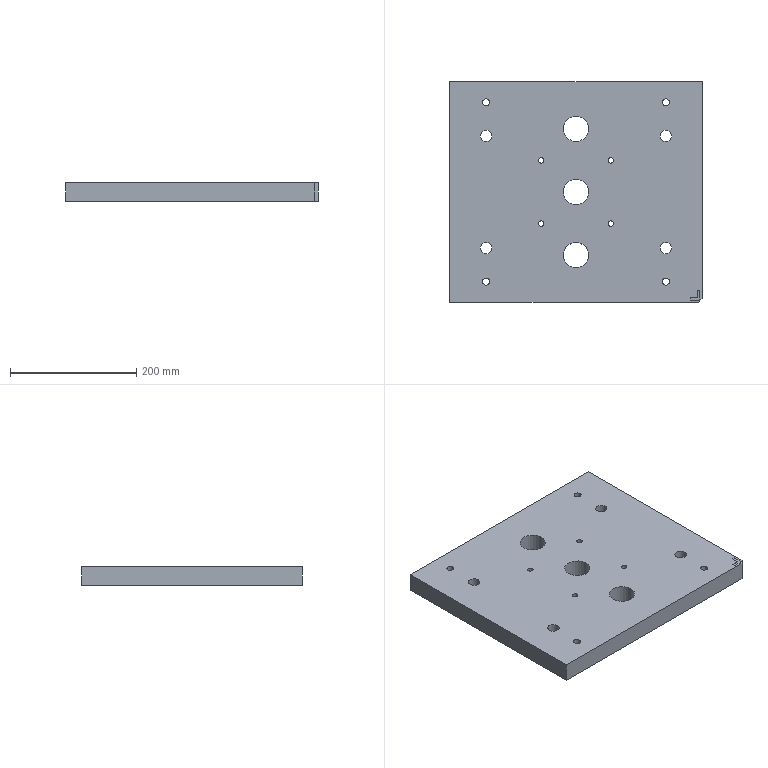Part | NX | features BD 2 | 1 solid | 56 faces | box 400 x 350 x 30 mm | volume 4007545 mm3 | cylinder 27 | plane 26 | cone 3 | commonest cylinder face diameters 18 x8 8.5 x4 11 x4 14 x4 26 x4 40 x3
STEP:
#1=CARTESIAN_POINT('',(48.,50.,-270.5));
#2=VERTEX_POINT('',#1);
#3=CARTESIAN_POINT('',(55.,50.,-270.5));
#4=DIRECTION('',(0.,0.,1.));
#5=DIRECTION('',(-1.,0.,0.));
#6=AXIS2_PLACEMENT_3D('',#3,#4,#5);
#7=CIRCLE('',#6,7.);
#8=EDGE_CURVE('',#2,#2,#7,.T.);
#9=ORIENTED_EDGE('',*,*,#8,.T.);
#10=EDGE_LOOP('',(#9));
#11=FACE_BOUND('',#10,.T.);
#12=CARTESIAN_POINT('',(-48.,-50.,-270.5));
#13=VERTEX_POINT('',#12);
#14=CARTESIAN_POINT('',(-55.,-50.,-270.5));
#15=DIRECTION('',(0.,0.,1.));
#16=DIRECTION('',(1.,0.,0.));
#17=AXIS2_PLACEMENT_3D('',#14,#15,#16);
#18=CIRCLE('',#17,7.);
#19=EDGE_CURVE('',#13,#13,#18,.T.);
#20=ORIENTED_EDGE('',*,*,#19,.T.);
#21=EDGE_LOOP('',(#20));
#22=FACE_BOUND('',#21,.T.);
#23=CARTESIAN_POINT('',(-21.,-100.,-270.5));
#24=VERTEX_POINT('',#23);
#25=CARTESIAN_POINT('',(0.,-100.,-270.5));
#26=DIRECTION('',(0.,0.,-1.));
#27=DIRECTION('',(-1.,0.,0.));
#28=AXIS2_PLACEMENT_3D('',#25,#26,#27);
#29=CIRCLE('',#28,21.);
#30=EDGE_CURVE('',#24,#24,#29,.F.);
#31=ORIENTED_EDGE('',*,*,#30,.T.);
#32=EDGE_LOOP('',(#31));
#33=FACE_BOUND('',#32,.T.);
#34=CARTESIAN_POINT('',(-21.,100.,-270.5));
#35=VERTEX_POINT('',#34);
#36=CARTESIAN_POINT('',(0.,100.,-270.5));
#37=DIRECTION('',(0.,0.,-1.));
#38=DIRECTION('',(-1.,0.,0.));
#39=AXIS2_PLACEMENT_3D('',#36,#37,#38);
#40=CIRCLE('',#39,21.);
#41=EDGE_CURVE('',#35,#35,#40,.F.);
#42=ORIENTED_EDGE('',*,*,#41,.T.);
#43=EDGE_LOOP('',(#42));
#44=FACE_BOUND('',#43,.T.);
#45=CARTESIAN_POINT('',(-21.,0.,-270.5));
#46=VERTEX_POINT('',#45);
#47=CARTESIAN_POINT('',(0.,0.,-270.5));
#48=DIRECTION('',(0.,0.,-1.));
#49=DIRECTION('',(-1.,0.,0.));
#50=AXIS2_PLACEMENT_3D('',#47,#48,#49);
#51=CIRCLE('',#50,21.);
#52=EDGE_CURVE('',#46,#46,#51,.F.);
#53=ORIENTED_EDGE('',*,*,#52,.T.);
#54=EDGE_LOOP('',(#53));
#55=FACE_BOUND('',#54,.T.);
#56=CARTESIAN_POINT('',(-151.5,-142.,-270.5));
#57=VERTEX_POINT('',#56);
#58=CARTESIAN_POINT('',(-142.5,-142.,-270.5));
#59=DIRECTION('',(0.,0.,1.));
#60=DIRECTION('',(-1.,0.,0.));
#61=AXIS2_PLACEMENT_3D('',#58,#59,#60);
#62=CIRCLE('',#61,9.);
#63=EDGE_CURVE('',#57,#57,#62,.T.);
#64=ORIENTED_EDGE('',*,*,#63,.T.);
#65=EDGE_LOOP('',(#64));
#66=FACE_BOUND('',#65,.T.);
#67=CARTESIAN_POINT('',(151.5,-142.,-270.5));
#68=VERTEX_POINT('',#67);
#69=CARTESIAN_POINT('',(142.5,-142.,-270.5));
#70=DIRECTION('',(0.,0.,1.));
#71=DIRECTION('',(1.,0.,0.));
#72=AXIS2_PLACEMENT_3D('',#69,#70,#71);
#73=CIRCLE('',#72,9.);
#74=EDGE_CURVE('',#68,#68,#73,.T.);
#75=ORIENTED_EDGE('',*,*,#74,.T.);
#76=EDGE_LOOP('',(#75));
#77=FACE_BOUND('',#76,.T.);
#78=CARTESIAN_POINT('',(-155.5,-89.,-270.5));
#79=VERTEX_POINT('',#78);
#80=CARTESIAN_POINT('',(-142.5,-89.,-270.5));
#81=DIRECTION('',(0.,0.,1.));
#82=DIRECTION('',(-1.,0.,0.));
#83=AXIS2_PLACEMENT_3D('',#80,#81,#82);
#84=CIRCLE('',#83,13.);
#85=EDGE_CURVE('',#79,#79,#84,.T.);
#86=ORIENTED_EDGE('',*,*,#85,.T.);
#87=EDGE_LOOP('',(#86));
#88=FACE_BOUND('',#87,.T.);
#89=CARTESIAN_POINT('',(155.5,89.,-270.5));
#90=VERTEX_POINT('',#89);
#91=CARTESIAN_POINT('',(142.5,89.,-270.5));
#92=DIRECTION('',(0.,0.,1.));
#93=DIRECTION('',(1.,0.,0.));
#94=AXIS2_PLACEMENT_3D('',#91,#92,#93);
#95=CIRCLE('',#94,13.);
#96=EDGE_CURVE('',#90,#90,#95,.T.);
#97=ORIENTED_EDGE('',*,*,#96,.T.);
#98=EDGE_LOOP('',(#97));
#99=FACE_BOUND('',#98,.T.);
#100=CARTESIAN_POINT('',(200.,-169.,-270.5));
#101=VERTEX_POINT('',#100);
#102=CARTESIAN_POINT('',(200.,175.,-270.5));
#103=VERTEX_POINT('',#102);
#104=CARTESIAN_POINT('',(200.,0.,-270.5));
#105=DIRECTION('',(0.,1.,0.));
#106=VECTOR('',#105,1000.);
#107=LINE('',#104,#106);
#108=EDGE_CURVE('',#101,#103,#107,.T.);
#109=ORIENTED_EDGE('',*,*,#108,.F.);
#110=CARTESIAN_POINT('',(194.,-175.,-270.5));
#111=VERTEX_POINT('',#110);
#112=CARTESIAN_POINT('',(184.5,-184.5,-270.5));
#113=DIRECTION('',(0.7071,0.7071,0.));
#114=VECTOR('',#113,1000.);
#115=LINE('',#112,#114);
#116=EDGE_CURVE('',#101,#111,#115,.F.);
#117=ORIENTED_EDGE('',*,*,#116,.T.);
#118=CARTESIAN_POINT('',(-200.,-175.,-270.5));
#119=VERTEX_POINT('',#118);
#120=CARTESIAN_POINT('',(0.,-175.,-270.5));
#121=DIRECTION('',(1.,0.,0.));
#122=VECTOR('',#121,1000.);
#123=LINE('',#120,#122);
#124=EDGE_CURVE('',#119,#111,#123,.T.);
#125=ORIENTED_EDGE('',*,*,#124,.F.);
#126=CARTESIAN_POINT('',(-200.,175.,-270.5));
#127=VERTEX_POINT('',#126);
#128=CARTESIAN_POINT('',(-200.,0.,-270.5));
#129=DIRECTION('',(0.,-1.,0.));
#130=VECTOR('',#129,1000.);
#131=LINE('',#128,#130);
#132=EDGE_CURVE('',#127,#119,#131,.T.);
#133=ORIENTED_EDGE('',*,*,#132,.F.);
#134=CARTESIAN_POINT('',(0.,175.,-270.5));
#135=DIRECTION('',(-1.,0.,0.));
#136=VECTOR('',#135,1000.);
#137=LINE('',#134,#136);
#138=EDGE_CURVE('',#103,#127,#137,.T.);
#139=ORIENTED_EDGE('',*,*,#138,.F.);
#140=EDGE_LOOP('',(#109,#117,#125,#133,#139));
#141=FACE_BOUND('',#140,.T.);
#142=CARTESIAN_POINT('',(155.5,-89.,-270.5));
#143=VERTEX_POINT('',#142);
#144=CARTESIAN_POINT('',(142.5,-89.,-270.5));
#145=DIRECTION('',(0.,0.,1.));
#146=DIRECTION('',(1.,0.,0.));
#147=AXIS2_PLACEMENT_3D('',#144,#145,#146);
#148=CIRCLE('',#147,13.);
#149=EDGE_CURVE('',#143,#143,#148,.T.);
#150=ORIENTED_EDGE('',*,*,#149,.T.);
#151=EDGE_LOOP('',(#150));
#152=FACE_BOUND('',#151,.T.);
#153=CARTESIAN_POINT('',(-129.5,89.,-270.5));
#154=VERTEX_POINT('',#153);
#155=CARTESIAN_POINT('',(-142.5,89.,-270.5));
#156=DIRECTION('',(0.,0.,1.));
#157=DIRECTION('',(1.,0.,0.));
#158=AXIS2_PLACEMENT_3D('',#155,#156,#157);
#159=CIRCLE('',#158,13.);
#160=EDGE_CURVE('',#154,#154,#159,.T.);
#161=ORIENTED_EDGE('',*,*,#160,.T.);
#162=EDGE_LOOP('',(#161));
#163=FACE_BOUND('',#162,.T.);
#164=CARTESIAN_POINT('',(151.5,142.,-270.5));
#165=VERTEX_POINT('',#164);
#166=CARTESIAN_POINT('',(142.5,142.,-270.5));
#167=DIRECTION('',(0.,0.,1.));
#168=DIRECTION('',(1.,0.,0.));
#169=AXIS2_PLACEMENT_3D('',#166,#167,#168);
#170=CIRCLE('',#169,9.);
#171=EDGE_CURVE('',#165,#165,#170,.T.);
#172=ORIENTED_EDGE('',*,*,#171,.T.);
#173=EDGE_LOOP('',(#172));
#174=FACE_BOUND('',#173,.T.);
#175=CARTESIAN_POINT('',(-133.5,142.,-270.5));
#176=VERTEX_POINT('',#175);
#177=CARTESIAN_POINT('',(-142.5,142.,-270.5));
#178=DIRECTION('',(0.,0.,1.));
#179=DIRECTION('',(1.,0.,0.));
#180=AXIS2_PLACEMENT_3D('',#177,#178,#179);
#181=CIRCLE('',#180,9.);
#182=EDGE_CURVE('',#176,#176,#181,.T.);
#183=ORIENTED_EDGE('',*,*,#182,.T.);
#184=EDGE_LOOP('',(#183));
#185=FACE_BOUND('',#184,.T.);
#186=CARTESIAN_POINT('',(62.,-50.,-270.5));
#187=VERTEX_POINT('',#186);
#188=CARTESIAN_POINT('',(55.,-50.,-270.5));
#189=DIRECTION('',(0.,0.,1.));
#190=DIRECTION('',(1.,0.,0.));
#191=AXIS2_PLACEMENT_3D('',#188,#189,#190);
#192=CIRCLE('',#191,7.);
#193=EDGE_CURVE('',#187,#187,#192,.T.);
#194=ORIENTED_EDGE('',*,*,#193,.T.);
#195=EDGE_LOOP('',(#194));
#196=FACE_BOUND('',#195,.T.);
#197=CARTESIAN_POINT('',(-48.,50.,-270.5));
#198=VERTEX_POINT('',#197);
#199=CARTESIAN_POINT('',(-55.,50.,-270.5));
#200=DIRECTION('',(0.,0.,1.));
#201=DIRECTION('',(1.,0.,0.));
#202=AXIS2_PLACEMENT_3D('',#199,#200,#201);
#203=CIRCLE('',#202,7.);
#204=EDGE_CURVE('',#198,#198,#203,.T.);
#205=ORIENTED_EDGE('',*,*,#204,.T.);
#206=EDGE_LOOP('',(#205));
#207=FACE_BOUND('',#206,.T.);
#208=CARTESIAN_POINT('',(0.,0.,-270.5));
#209=DIRECTION('',(0.,0.,-1.));
#210=DIRECTION('',(-1.,0.,0.));
#211=AXIS2_PLACEMENT_3D('',#208,#209,#210);
#212=PLANE('',#211);
#213=ADVANCED_FACE('',(#11,#22,#33,#44,#55,#66,#77,#88,#99,#141,#152,#163,#174,#185,#196,#207),#212,.T.);
#214=CARTESIAN_POINT('',(50.75,50.,-240.5));
#215=VERTEX_POINT('',#214);
#216=CARTESIAN_POINT('',(55.,50.,-240.5));
#217=DIRECTION('',(0.,0.,-1.));
#218=DIRECTION('',(-1.,0.,0.));
#219=AXIS2_PLACEMENT_3D('',#216,#217,#218);
#220=CIRCLE('',#219,4.25);
#221=EDGE_CURVE('',#215,#215,#220,.T.);
#222=ORIENTED_EDGE('',*,*,#221,.T.);
#223=EDGE_LOOP('',(#222));
#224=FACE_BOUND('',#223,.T.);
#225=CARTESIAN_POINT('',(-50.75,-50.,-240.5));
#226=VERTEX_POINT('',#225);
#227=CARTESIAN_POINT('',(-55.,-50.,-240.5));
#228=DIRECTION('',(0.,0.,-1.));
#229=DIRECTION('',(1.,0.,0.));
#230=AXIS2_PLACEMENT_3D('',#227,#228,#229);
#231=CIRCLE('',#230,4.25);
#232=EDGE_CURVE('',#226,#226,#231,.T.);
#233=ORIENTED_EDGE('',*,*,#232,.T.);
#234=EDGE_LOOP('',(#233));
#235=FACE_BOUND('',#234,.T.);
#236=CARTESIAN_POINT('',(20.,-100.,-240.5));
#237=VERTEX_POINT('',#236);
#238=CARTESIAN_POINT('',(0.,-100.,-240.5));
#239=DIRECTION('',(0.,0.,1.));
#240=DIRECTION('',(1.,0.,0.));
#241=AXIS2_PLACEMENT_3D('',#238,#239,#240);
#242=CIRCLE('',#241,20.);
#243=EDGE_CURVE('',#237,#237,#242,.T.);
#244=ORIENTED_EDGE('',*,*,#243,.F.);
#245=EDGE_LOOP('',(#244));
#246=FACE_BOUND('',#245,.T.);
#247=CARTESIAN_POINT('',(20.,100.,-240.5));
#248=VERTEX_POINT('',#247);
#249=CARTESIAN_POINT('',(0.,100.,-240.5));
#250=DIRECTION('',(0.,0.,1.));
#251=DIRECTION('',(1.,0.,0.));
#252=AXIS2_PLACEMENT_3D('',#249,#250,#251);
#253=CIRCLE('',#252,20.);
#254=EDGE_CURVE('',#248,#248,#253,.T.);
#255=ORIENTED_EDGE('',*,*,#254,.F.);
#256=EDGE_LOOP('',(#255));
#257=FACE_BOUND('',#256,.T.);
#258=CARTESIAN_POINT('',(-148.,-142.,-240.5));
#259=VERTEX_POINT('',#258);
#260=CARTESIAN_POINT('',(-142.5,-142.,-240.5));
#261=DIRECTION('',(0.,0.,-1.));
#262=DIRECTION('',(-1.,0.,0.));
#263=AXIS2_PLACEMENT_3D('',#260,#261,#262);
#264=CIRCLE('',#263,5.5);
#265=EDGE_CURVE('',#259,#259,#264,.T.);
#266=ORIENTED_EDGE('',*,*,#265,.T.);
#267=EDGE_LOOP('',(#266));
#268=FACE_BOUND('',#267,.T.);
#269=CARTESIAN_POINT('',(148.,-142.,-240.5));
#270=VERTEX_POINT('',#269);
#271=CARTESIAN_POINT('',(142.5,-142.,-240.5));
#272=DIRECTION('',(0.,0.,-1.));
#273=DIRECTION('',(1.,0.,0.));
#274=AXIS2_PLACEMENT_3D('',#271,#272,#273);
#275=CIRCLE('',#274,5.5);
#276=EDGE_CURVE('',#270,#270,#275,.T.);
#277=ORIENTED_EDGE('',*,*,#276,.T.);
#278=EDGE_LOOP('',(#277));
#279=FACE_BOUND('',#278,.T.);
#280=CARTESIAN_POINT('',(-151.5,-89.,-240.5));
#281=VERTEX_POINT('',#280);
#282=CARTESIAN_POINT('',(-142.5,-89.,-240.5));
#283=DIRECTION('',(0.,0.,-1.));
#284=DIRECTION('',(-1.,0.,0.));
#285=AXIS2_PLACEMENT_3D('',#282,#283,#284);
#286=CIRCLE('',#285,9.);
#287=EDGE_CURVE('',#281,#281,#286,.T.);
#288=ORIENTED_EDGE('',*,*,#287,.T.);
#289=EDGE_LOOP('',(#288));
#290=FACE_BOUND('',#289,.T.);
#291=CARTESIAN_POINT('',(151.5,89.,-240.5));
#292=VERTEX_POINT('',#291);
#293=CARTESIAN_POINT('',(142.5,89.,-240.5));
#294=DIRECTION('',(0.,0.,-1.));
#295=DIRECTION('',(1.,0.,0.));
#296=AXIS2_PLACEMENT_3D('',#293,#294,#295);
#297=CIRCLE('',#296,9.);
#298=EDGE_CURVE('',#292,#292,#297,.T.);
#299=ORIENTED_EDGE('',*,*,#298,.T.);
#300=EDGE_LOOP('',(#299));
#301=FACE_BOUND('',#300,.T.);
#302=CARTESIAN_POINT('',(192.5,-156.25,-240.5));
#303=VERTEX_POINT('',#302);
#304=CARTESIAN_POINT('',(192.5,-167.5,-240.5));
#305=VERTEX_POINT('',#304);
#306=CARTESIAN_POINT('',(192.5,-161.875,-240.5));
#307=DIRECTION('',(0.,-1.,0.));
#308=VECTOR('',#307,1000.);
#309=LINE('',#306,#308);
#310=EDGE_CURVE('',#303,#305,#309,.T.);
#311=ORIENTED_EDGE('',*,*,#310,.F.);
#312=CARTESIAN_POINT('',(196.25,-156.25,-240.5));
#313=VERTEX_POINT('',#312);
#314=CARTESIAN_POINT('',(188.75,-156.25,-240.5));
#315=DIRECTION('',(1.,0.,0.));
#316=VECTOR('',#315,1000.);
#317=LINE('',#314,#316);
#318=EDGE_CURVE('',#303,#313,#317,.T.);
#319=ORIENTED_EDGE('',*,*,#318,.T.);
#320=CARTESIAN_POINT('',(196.25,-171.25,-240.5));
#321=VERTEX_POINT('',#320);
#322=CARTESIAN_POINT('',(196.25,-163.75,-240.5));
#323=DIRECTION('',(0.,-1.,0.));
#324=VECTOR('',#323,1000.);
#325=LINE('',#322,#324);
#326=EDGE_CURVE('',#313,#321,#325,.T.);
#327=ORIENTED_EDGE('',*,*,#326,.T.);
#328=CARTESIAN_POINT('',(181.25,-171.25,-240.5));
#329=VERTEX_POINT('',#328);
#330=CARTESIAN_POINT('',(188.75,-171.25,-240.5));
#331=DIRECTION('',(-1.,0.,0.));
#332=VECTOR('',#331,1000.);
#333=LINE('',#330,#332);
#334=EDGE_CURVE('',#321,#329,#333,.T.);
#335=ORIENTED_EDGE('',*,*,#334,.T.);
#336=CARTESIAN_POINT('',(181.25,-167.5,-240.5));
#337=VERTEX_POINT('',#336);
#338=CARTESIAN_POINT('',(181.25,-163.75,-240.5));
#339=DIRECTION('',(0.,1.,0.));
#340=VECTOR('',#339,1000.);
#341=LINE('',#338,#340);
#342=EDGE_CURVE('',#329,#337,#341,.T.);
#343=ORIENTED_EDGE('',*,*,#342,.T.);
#344=CARTESIAN_POINT('',(186.875,-167.5,-240.5));
#345=DIRECTION('',(-1.,0.,0.));
#346=VECTOR('',#345,1000.);
#347=LINE('',#344,#346);
#348=EDGE_CURVE('',#305,#337,#347,.T.);
#349=ORIENTED_EDGE('',*,*,#348,.F.);
#350=EDGE_LOOP('',(#311,#319,#327,#335,#343,#349));
#351=FACE_BOUND('',#350,.T.);
#352=CARTESIAN_POINT('',(194.,-175.,-240.5));
#353=VERTEX_POINT('',#352);
#354=CARTESIAN_POINT('',(-200.,-175.,-240.5));
#355=VERTEX_POINT('',#354);
#356=CARTESIAN_POINT('',(0.,-175.,-240.5));
#357=DIRECTION('',(-1.,0.,0.));
#358=VECTOR('',#357,1000.);
#359=LINE('',#356,#358);
#360=EDGE_CURVE('',#353,#355,#359,.T.);
#361=ORIENTED_EDGE('',*,*,#360,.F.);
#362=CARTESIAN_POINT('',(200.,-169.,-240.5));
#363=VERTEX_POINT('',#362);
#364=CARTESIAN_POINT('',(184.5,-184.5,-240.5));
#365=DIRECTION('',(-0.7071,-0.7071,0.));
#366=VECTOR('',#365,1000.);
#367=LINE('',#364,#366);
#368=EDGE_CURVE('',#353,#363,#367,.F.);
#369=ORIENTED_EDGE('',*,*,#368,.T.);
#370=CARTESIAN_POINT('',(200.,175.,-240.5));
#371=VERTEX_POINT('',#370);
#372=CARTESIAN_POINT('',(200.,0.,-240.5));
#373=DIRECTION('',(0.,-1.,0.));
#374=VECTOR('',#373,1000.);
#375=LINE('',#372,#374);
#376=EDGE_CURVE('',#371,#363,#375,.T.);
#377=ORIENTED_EDGE('',*,*,#376,.F.);
#378=CARTESIAN_POINT('',(-200.,175.,-240.5));
#379=VERTEX_POINT('',#378);
#380=CARTESIAN_POINT('',(0.,175.,-240.5));
#381=DIRECTION('',(1.,0.,0.));
#382=VECTOR('',#381,1000.);
#383=LINE('',#380,#382);
#384=EDGE_CURVE('',#379,#371,#383,.T.);
#385=ORIENTED_EDGE('',*,*,#384,.F.);
#386=CARTESIAN_POINT('',(-200.,0.,-240.5));
#387=DIRECTION('',(0.,1.,0.));
#388=VECTOR('',#387,1000.);
#389=LINE('',#386,#388);
#390=EDGE_CURVE('',#355,#379,#389,.T.);
#391=ORIENTED_EDGE('',*,*,#390,.F.);
#392=EDGE_LOOP('',(#361,#369,#377,#385,#391));
#393=FACE_BOUND('',#392,.T.);
#394=CARTESIAN_POINT('',(151.5,-89.,-240.5));
#395=VERTEX_POINT('',#394);
#396=CARTESIAN_POINT('',(142.5,-89.,-240.5));
#397=DIRECTION('',(0.,0.,-1.));
#398=DIRECTION('',(1.,0.,0.));
#399=AXIS2_PLACEMENT_3D('',#396,#397,#398);
#400=CIRCLE('',#399,9.);
#401=EDGE_CURVE('',#395,#395,#400,.T.);
#402=ORIENTED_EDGE('',*,*,#401,.T.);
#403=EDGE_LOOP('',(#402));
#404=FACE_BOUND('',#403,.T.);
#405=CARTESIAN_POINT('',(-133.5,89.,-240.5));
#406=VERTEX_POINT('',#405);
#407=CARTESIAN_POINT('',(-142.5,89.,-240.5));
#408=DIRECTION('',(0.,0.,-1.));
#409=DIRECTION('',(1.,0.,0.));
#410=AXIS2_PLACEMENT_3D('',#407,#408,#409);
#411=CIRCLE('',#410,9.);
#412=EDGE_CURVE('',#406,#406,#411,.T.);
#413=ORIENTED_EDGE('',*,*,#412,.T.);
#414=EDGE_LOOP('',(#413));
#415=FACE_BOUND('',#414,.T.);
#416=CARTESIAN_POINT('',(148.,142.,-240.5));
#417=VERTEX_POINT('',#416);
#418=CARTESIAN_POINT('',(142.5,142.,-240.5));
#419=DIRECTION('',(0.,0.,-1.));
#420=DIRECTION('',(1.,0.,0.));
#421=AXIS2_PLACEMENT_3D('',#418,#419,#420);
#422=CIRCLE('',#421,5.5);
#423=EDGE_CURVE('',#417,#417,#422,.T.);
#424=ORIENTED_EDGE('',*,*,#423,.T.);
#425=EDGE_LOOP('',(#424));
#426=FACE_BOUND('',#425,.T.);
#427=CARTESIAN_POINT('',(-137.,142.,-240.5));
#428=VERTEX_POINT('',#427);
#429=CARTESIAN_POINT('',(-142.5,142.,-240.5));
#430=DIRECTION('',(0.,0.,-1.));
#431=DIRECTION('',(1.,0.,0.));
#432=AXIS2_PLACEMENT_3D('',#429,#430,#431);
#433=CIRCLE('',#432,5.5);
#434=EDGE_CURVE('',#428,#428,#433,.T.);
#435=ORIENTED_EDGE('',*,*,#434,.T.);
#436=EDGE_LOOP('',(#435));
#437=FACE_BOUND('',#436,.T.);
#438=CARTESIAN_POINT('',(20.,0.,-240.5));
#439=VERTEX_POINT('',#438);
#440=CARTESIAN_POINT('',(0.,0.,-240.5));
#441=DIRECTION('',(0.,0.,1.));
#442=DIRECTION('',(1.,0.,0.));
#443=AXIS2_PLACEMENT_3D('',#440,#441,#442);
#444=CIRCLE('',#443,20.);
#445=EDGE_CURVE('',#439,#439,#444,.F.);
#446=ORIENTED_EDGE('',*,*,#445,.T.);
#447=EDGE_LOOP('',(#446));
#448=FACE_BOUND('',#447,.T.);
#449=CARTESIAN_POINT('',(59.25,-50.,-240.5));
#450=VERTEX_POINT('',#449);
#451=CARTESIAN_POINT('',(55.,-50.,-240.5));
#452=DIRECTION('',(0.,0.,-1.));
#453=DIRECTION('',(1.,0.,0.));
#454=AXIS2_PLACEMENT_3D('',#451,#452,#453);
#455=CIRCLE('',#454,4.25);
#456=EDGE_CURVE('',#450,#450,#455,.T.);
#457=ORIENTED_EDGE('',*,*,#456,.T.);
#458=EDGE_LOOP('',(#457));
#459=FACE_BOUND('',#458,.T.);
#460=CARTESIAN_POINT('',(-50.75,50.,-240.5));
#461=VERTEX_POINT('',#460);
#462=CARTESIAN_POINT('',(-55.,50.,-240.5));
#463=DIRECTION('',(0.,0.,-1.));
#464=DIRECTION('',(1.,0.,0.));
#465=AXIS2_PLACEMENT_3D('',#462,#463,#464);
#466=CIRCLE('',#465,4.25);
#467=EDGE_CURVE('',#461,#461,#466,.T.);
#468=ORIENTED_EDGE('',*,*,#467,.T.);
#469=EDGE_LOOP('',(#468));
#470=FACE_BOUND('',#469,.T.);
#471=CARTESIAN_POINT('',(0.,0.,-240.5));
#472=DIRECTION('',(0.,0.,1.));
#473=DIRECTION('',(1.,0.,0.));
#474=AXIS2_PLACEMENT_3D('',#471,#472,#473);
#475=PLANE('',#474);
#476=ADVANCED_FACE('',(#224,#235,#246,#257,#268,#279,#290,#301,#351,#393,#404,#415,#426,#437,#448,#459,#470),#475,.T.);
#477=CARTESIAN_POINT('',(-20.,-100.,-269.5));
#478=VERTEX_POINT('',#477);
#479=CARTESIAN_POINT('',(0.,-100.,-269.5));
#480=DIRECTION('',(0.,0.,-1.));
#481=DIRECTION('',(-1.,0.,0.));
#482=AXIS2_PLACEMENT_3D('',#479,#480,#481);
#483=CIRCLE('',#482,20.);
#484=EDGE_CURVE('',#478,#478,#483,.T.);
#485=ORIENTED_EDGE('',*,*,#484,.T.);
#486=EDGE_LOOP('',(#485));
#487=FACE_BOUND('',#486,.T.);
#488=ORIENTED_EDGE('',*,*,#243,.T.);
#489=EDGE_LOOP('',(#488));
#490=FACE_BOUND('',#489,.T.);
#491=CARTESIAN_POINT('',(0.,-100.,-270.5));
#492=DIRECTION('',(0.,0.,1.));
#493=DIRECTION('',(1.,0.,0.));
#494=AXIS2_PLACEMENT_3D('',#491,#492,#493);
#495=CYLINDRICAL_SURFACE('',#494,20.);
#496=ADVANCED_FACE('',(#487,#490),#495,.F.);
#497=CARTESIAN_POINT('',(192.5,-167.5,-240.6));
#498=VERTEX_POINT('',#497);
#499=CARTESIAN_POINT('',(181.25,-167.5,-240.6));
#500=VERTEX_POINT('',#499);
#501=CARTESIAN_POINT('',(186.875,-167.5,-240.6));
#502=DIRECTION('',(1.,0.,0.));
#503=VECTOR('',#502,1000.);
#504=LINE('',#501,#503);
#505=EDGE_CURVE('',#498,#500,#504,.F.);
#506=ORIENTED_EDGE('',*,*,#505,.T.);
#507=CARTESIAN_POINT('',(181.25,-171.25,-240.6));
#508=VERTEX_POINT('',#507);
#509=CARTESIAN_POINT('',(181.25,-163.75,-240.6));
#510=DIRECTION('',(0.,-1.,0.));
#511=VECTOR('',#510,1000.);
#512=LINE('',#509,#511);
#513=EDGE_CURVE('',#508,#500,#512,.F.);
#514=ORIENTED_EDGE('',*,*,#513,.F.);
#515=CARTESIAN_POINT('',(196.25,-171.25,-240.6));
#516=VERTEX_POINT('',#515);
#517=CARTESIAN_POINT('',(188.75,-171.25,-240.6));
#518=DIRECTION('',(1.,0.,0.));
#519=VECTOR('',#518,1000.);
#520=LINE('',#517,#519);
#521=EDGE_CURVE('',#516,#508,#520,.F.);
#522=ORIENTED_EDGE('',*,*,#521,.F.);
#523=CARTESIAN_POINT('',(196.25,-156.25,-240.6));
#524=VERTEX_POINT('',#523);
#525=CARTESIAN_POINT('',(196.25,-163.75,-240.6));
#526=DIRECTION('',(0.,1.,0.));
#527=VECTOR('',#526,1000.);
#528=LINE('',#525,#527);
#529=EDGE_CURVE('',#524,#516,#528,.F.);
#530=ORIENTED_EDGE('',*,*,#529,.F.);
#531=CARTESIAN_POINT('',(192.5,-156.25,-240.6));
#532=VERTEX_POINT('',#531);
#533=CARTESIAN_POINT('',(188.75,-156.25,-240.6));
#534=DIRECTION('',(-1.,0.,0.));
#535=VECTOR('',#534,1000.);
#536=LINE('',#533,#535);
#537=EDGE_CURVE('',#532,#524,#536,.F.);
#538=ORIENTED_EDGE('',*,*,#537,.F.);
#539=CARTESIAN_POINT('',(192.5,-161.875,-240.6));
#540=DIRECTION('',(0.,1.,0.));
#541=VECTOR('',#540,1000.);
#542=LINE('',#539,#541);
#543=EDGE_CURVE('',#532,#498,#542,.F.);
#544=ORIENTED_EDGE('',*,*,#543,.T.);
#545=EDGE_LOOP('',(#506,#514,#522,#530,#538,#544));
#546=FACE_BOUND('',#545,.T.);
#547=CARTESIAN_POINT('',(188.75,-163.75,-240.6));
#548=DIRECTION('',(0.,0.,-1.));
#549=DIRECTION('',(-1.,0.,0.));
#550=AXIS2_PLACEMENT_3D('',#547,#548,#549);
#551=PLANE('',#550);
#552=ADVANCED_FACE('',(#546),#551,.F.);
#553=CARTESIAN_POINT('',(-137.,142.,-259.5));
#554=VERTEX_POINT('',#553);
#555=CARTESIAN_POINT('',(-142.5,142.,-259.5));
#556=DIRECTION('',(0.,0.,1.));
#557=DIRECTION('',(1.,0.,0.));
#558=AXIS2_PLACEMENT_3D('',#555,#556,#557);
#559=CIRCLE('',#558,5.5);
#560=EDGE_CURVE('',#554,#554,#559,.T.);
#561=ORIENTED_EDGE('',*,*,#560,.T.);
#562=EDGE_LOOP('',(#561));
#563=FACE_BOUND('',#562,.T.);
#564=CARTESIAN_POINT('',(-133.5,142.,-259.5));
#565=VERTEX_POINT('',#564);
#566=CARTESIAN_POINT('',(-142.5,142.,-259.5));
#567=DIRECTION('',(0.,0.,-1.));
#568=DIRECTION('',(1.,0.,0.));
#569=AXIS2_PLACEMENT_3D('',#566,#567,#568);
#570=CIRCLE('',#569,9.);
#571=EDGE_CURVE('',#565,#565,#570,.F.);
#572=ORIENTED_EDGE('',*,*,#571,.F.);
#573=EDGE_LOOP('',(#572));
#574=FACE_BOUND('',#573,.T.);
#575=CARTESIAN_POINT('',(-142.5,142.,-259.5));
#576=DIRECTION('',(0.,0.,1.));
#577=DIRECTION('',(1.,0.,0.));
#578=AXIS2_PLACEMENT_3D('',#575,#576,#577);
#579=PLANE('',#578);
#580=ADVANCED_FACE('',(#563,#574),#579,.F.);
#581=CARTESIAN_POINT('',(148.,142.,-259.5));
#582=VERTEX_POINT('',#581);
#583=CARTESIAN_POINT('',(142.5,142.,-259.5));
#584=DIRECTION('',(0.,0.,1.));
#585=DIRECTION('',(1.,0.,0.));
#586=AXIS2_PLACEMENT_3D('',#583,#584,#585);
#587=CIRCLE('',#586,5.5);
#588=EDGE_CURVE('',#582,#582,#587,.T.);
#589=ORIENTED_EDGE('',*,*,#588,.T.);
#590=EDGE_LOOP('',(#589));
#591=FACE_BOUND('',#590,.T.);
#592=CARTESIAN_POINT('',(151.5,142.,-259.5));
#593=VERTEX_POINT('',#592);
#594=CARTESIAN_POINT('',(142.5,142.,-259.5));
#595=DIRECTION('',(0.,0.,-1.));
#596=DIRECTION('',(1.,0.,0.));
#597=AXIS2_PLACEMENT_3D('',#594,#595,#596);
#598=CIRCLE('',#597,9.);
#599=EDGE_CURVE('',#593,#593,#598,.F.);
#600=ORIENTED_EDGE('',*,*,#599,.F.);
#601=EDGE_LOOP('',(#600));
#602=FACE_BOUND('',#601,.T.);
#603=CARTESIAN_POINT('',(142.5,142.,-259.5));
#604=DIRECTION('',(0.,0.,1.));
#605=DIRECTION('',(1.,0.,0.));
#606=AXIS2_PLACEMENT_3D('',#603,#604,#605);
#607=PLANE('',#606);
#608=ADVANCED_FACE('',(#591,#602),#607,.F.);
#609=CARTESIAN_POINT('',(-133.5,89.,-253.));
#610=VERTEX_POINT('',#609);
#611=CARTESIAN_POINT('',(-142.5,89.,-253.));
#612=DIRECTION('',(0.,0.,1.));
#613=DIRECTION('',(1.,0.,0.));
#614=AXIS2_PLACEMENT_3D('',#611,#612,#613);
#615=CIRCLE('',#614,9.);
#616=EDGE_CURVE('',#610,#610,#615,.T.);
#617=ORIENTED_EDGE('',*,*,#616,.T.);
#618=EDGE_LOOP('',(#617));
#619=FACE_BOUND('',#618,.T.);
#620=CARTESIAN_POINT('',(-129.5,89.,-253.));
#621=VERTEX_POINT('',#620);
#622=CARTESIAN_POINT('',(-142.5,89.,-253.));
#623=DIRECTION('',(0.,0.,-1.));
#624=DIRECTION('',(1.,0.,0.));
#625=AXIS2_PLACEMENT_3D('',#622,#623,#624);
#626=CIRCLE('',#625,13.);
#627=EDGE_CURVE('',#621,#621,#626,.F.);
#628=ORIENTED_EDGE('',*,*,#627,.F.);
#629=EDGE_LOOP('',(#628));
#630=FACE_BOUND('',#629,.T.);
#631=CARTESIAN_POINT('',(-142.5,89.,-253.));
#632=DIRECTION('',(0.,0.,1.));
#633=DIRECTION('',(1.,0.,0.));
#634=AXIS2_PLACEMENT_3D('',#631,#632,#633);
#635=PLANE('',#634);
#636=ADVANCED_FACE('',(#619,#630),#635,.F.);
#637=CARTESIAN_POINT('',(151.5,-89.,-253.));
#638=VERTEX_POINT('',#637);
#639=CARTESIAN_POINT('',(142.5,-89.,-253.));
#640=DIRECTION('',(0.,0.,1.));
#641=DIRECTION('',(1.,0.,0.));
#642=AXIS2_PLACEMENT_3D('',#639,#640,#641);
#643=CIRCLE('',#642,9.);
#644=EDGE_CURVE('',#638,#638,#643,.T.);
#645=ORIENTED_EDGE('',*,*,#644,.T.);
#646=EDGE_LOOP('',(#645));
#647=FACE_BOUND('',#646,.T.);
#648=CARTESIAN_POINT('',(155.5,-89.,-253.));
#649=VERTEX_POINT('',#648);
#650=CARTESIAN_POINT('',(142.5,-89.,-253.));
#651=DIRECTION('',(0.,0.,-1.));
#652=DIRECTION('',(1.,0.,0.));
#653=AXIS2_PLACEMENT_3D('',#650,#651,#652);
#654=CIRCLE('',#653,13.);
#655=EDGE_CURVE('',#649,#649,#654,.F.);
#656=ORIENTED_EDGE('',*,*,#655,.F.);
#657=EDGE_LOOP('',(#656));
#658=FACE_BOUND('',#657,.T.);
#659=CARTESIAN_POINT('',(142.5,-89.,-253.));
#660=DIRECTION('',(0.,0.,1.));
#661=DIRECTION('',(1.,0.,0.));
#662=AXIS2_PLACEMENT_3D('',#659,#660,#661);
#663=PLANE('',#662);
#664=ADVANCED_FACE('',(#647,#658),#663,.F.);
#665=CARTESIAN_POINT('',(151.5,89.,-253.));
#666=VERTEX_POINT('',#665);
#667=CARTESIAN_POINT('',(142.5,89.,-253.));
#668=DIRECTION('',(0.,0.,1.));
#669=DIRECTION('',(1.,0.,0.));
#670=AXIS2_PLACEMENT_3D('',#667,#668,#669);
#671=CIRCLE('',#670,9.);
#672=EDGE_CURVE('',#666,#666,#671,.T.);
#673=ORIENTED_EDGE('',*,*,#672,.T.);
#674=EDGE_LOOP('',(#673));
#675=FACE_BOUND('',#674,.T.);
#676=CARTESIAN_POINT('',(155.5,89.,-253.));
#677=VERTEX_POINT('',#676);
#678=CARTESIAN_POINT('',(142.5,89.,-253.));
#679=DIRECTION('',(0.,0.,-1.));
#680=DIRECTION('',(1.,0.,0.));
#681=AXIS2_PLACEMENT_3D('',#678,#679,#680);
#682=CIRCLE('',#681,13.);
#683=EDGE_CURVE('',#677,#677,#682,.F.);
#684=ORIENTED_EDGE('',*,*,#683,.F.);
#685=EDGE_LOOP('',(#684));
#686=FACE_BOUND('',#685,.T.);
#687=CARTESIAN_POINT('',(142.5,89.,-253.));
#688=DIRECTION('',(0.,0.,1.));
#689=DIRECTION('',(1.,0.,0.));
#690=AXIS2_PLACEMENT_3D('',#687,#688,#689);
#691=PLANE('',#690);
#692=ADVANCED_FACE('',(#675,#686),#691,.F.);
#693=CARTESIAN_POINT('',(-151.5,-89.,-253.));
#694=VERTEX_POINT('',#693);
#695=CARTESIAN_POINT('',(-142.5,-89.,-253.));
#696=DIRECTION('',(0.,0.,1.));
#697=DIRECTION('',(-1.,0.,0.));
#698=AXIS2_PLACEMENT_3D('',#695,#696,#697);
#699=CIRCLE('',#698,9.);
#700=EDGE_CURVE('',#694,#694,#699,.T.);
#701=ORIENTED_EDGE('',*,*,#700,.T.);
#702=EDGE_LOOP('',(#701));
#703=FACE_BOUND('',#702,.T.);
#704=CARTESIAN_POINT('',(-155.5,-89.,-253.));
#705=VERTEX_POINT('',#704);
#706=CARTESIAN_POINT('',(-142.5,-89.,-253.));
#707=DIRECTION('',(0.,0.,-1.));
#708=DIRECTION('',(-1.,0.,0.));
#709=AXIS2_PLACEMENT_3D('',#706,#707,#708);
#710=CIRCLE('',#709,13.);
#711=EDGE_CURVE('',#705,#705,#710,.F.);
#712=ORIENTED_EDGE('',*,*,#711,.F.);
#713=EDGE_LOOP('',(#712));
#714=FACE_BOUND('',#713,.T.);
#715=CARTESIAN_POINT('',(-142.5,-89.,-253.));
#716=DIRECTION('',(0.,0.,1.));
#717=DIRECTION('',(-1.,0.,0.));
#718=AXIS2_PLACEMENT_3D('',#715,#716,#717);
#719=PLANE('',#718);
#720=ADVANCED_FACE('',(#703,#714),#719,.F.);
#721=CARTESIAN_POINT('',(148.,-142.,-259.5));
#722=VERTEX_POINT('',#721);
#723=CARTESIAN_POINT('',(142.5,-142.,-259.5));
#724=DIRECTION('',(0.,0.,1.));
#725=DIRECTION('',(1.,0.,0.));
#726=AXIS2_PLACEMENT_3D('',#723,#724,#725);
#727=CIRCLE('',#726,5.5);
#728=EDGE_CURVE('',#722,#722,#727,.T.);
#729=ORIENTED_EDGE('',*,*,#728,.T.);
#730=EDGE_LOOP('',(#729));
#731=FACE_BOUND('',#730,.T.);
#732=CARTESIAN_POINT('',(151.5,-142.,-259.5));
#733=VERTEX_POINT('',#732);
#734=CARTESIAN_POINT('',(142.5,-142.,-259.5));
#735=DIRECTION('',(0.,0.,-1.));
#736=DIRECTION('',(1.,0.,0.));
#737=AXIS2_PLACEMENT_3D('',#734,#735,#736);
#738=CIRCLE('',#737,9.);
#739=EDGE_CURVE('',#733,#733,#738,.F.);
#740=ORIENTED_EDGE('',*,*,#739,.F.);
#741=EDGE_LOOP('',(#740));
#742=FACE_BOUND('',#741,.T.);
#743=CARTESIAN_POINT('',(142.5,-142.,-259.5));
#744=DIRECTION('',(0.,0.,1.));
#745=DIRECTION('',(1.,0.,0.));
#746=AXIS2_PLACEMENT_3D('',#743,#744,#745);
#747=PLANE('',#746);
#748=ADVANCED_FACE('',(#731,#742),#747,.F.);
#749=CARTESIAN_POINT('',(-148.,-142.,-259.5));
#750=VERTEX_POINT('',#749);
#751=CARTESIAN_POINT('',(-142.5,-142.,-259.5));
#752=DIRECTION('',(0.,0.,1.));
#753=DIRECTION('',(-1.,0.,0.));
#754=AXIS2_PLACEMENT_3D('',#751,#752,#753);
#755=CIRCLE('',#754,5.5);
#756=EDGE_CURVE('',#750,#750,#755,.T.);
#757=ORIENTED_EDGE('',*,*,#756,.T.);
#758=EDGE_LOOP('',(#757));
#759=FACE_BOUND('',#758,.T.);
#760=CARTESIAN_POINT('',(-151.5,-142.,-259.5));
#761=VERTEX_POINT('',#760);
#762=CARTESIAN_POINT('',(-142.5,-142.,-259.5));
#763=DIRECTION('',(0.,0.,-1.));
#764=DIRECTION('',(-1.,0.,0.));
#765=AXIS2_PLACEMENT_3D('',#762,#763,#764);
#766=CIRCLE('',#765,9.);
#767=EDGE_CURVE('',#761,#761,#766,.F.);
#768=ORIENTED_EDGE('',*,*,#767,.F.);
#769=EDGE_LOOP('',(#768));
#770=FACE_BOUND('',#769,.T.);
#771=CARTESIAN_POINT('',(-142.5,-142.,-259.5));
#772=DIRECTION('',(0.,0.,1.));
#773=DIRECTION('',(-1.,0.,0.));
#774=AXIS2_PLACEMENT_3D('',#771,#772,#773);
#775=PLANE('',#774);
#776=ADVANCED_FACE('',(#759,#770),#775,.F.);
#777=CARTESIAN_POINT('',(-20.,0.,-269.5));
#778=VERTEX_POINT('',#777);
#779=CARTESIAN_POINT('',(0.,0.,-269.5));
#780=DIRECTION('',(0.,0.,-1.));
#781=DIRECTION('',(-1.,0.,0.));
#782=AXIS2_PLACEMENT_3D('',#779,#780,#781);
#783=CIRCLE('',#782,20.);
#784=EDGE_CURVE('',#778,#778,#783,.T.);
#785=ORIENTED_EDGE('',*,*,#784,.T.);
#786=EDGE_LOOP('',(#785));
#787=FACE_BOUND('',#786,.T.);
#788=ORIENTED_EDGE('',*,*,#445,.F.);
#789=EDGE_LOOP('',(#788));
#790=FACE_BOUND('',#789,.T.);
#791=CARTESIAN_POINT('',(0.,0.,-270.5));
#792=DIRECTION('',(0.,0.,1.));
#793=DIRECTION('',(1.,0.,0.));
#794=AXIS2_PLACEMENT_3D('',#791,#792,#793);
#795=CYLINDRICAL_SURFACE('',#794,20.);
#796=ADVANCED_FACE('',(#787,#790),#795,.F.);
#797=ORIENTED_EDGE('',*,*,#560,.F.);
#798=EDGE_LOOP('',(#797));
#799=FACE_BOUND('',#798,.T.);
#800=ORIENTED_EDGE('',*,*,#434,.F.);
#801=EDGE_LOOP('',(#800));
#802=FACE_BOUND('',#801,.T.);
#803=CARTESIAN_POINT('',(-142.5,142.,-270.5));
#804=DIRECTION('',(0.,0.,1.));
#805=DIRECTION('',(1.,0.,0.));
#806=AXIS2_PLACEMENT_3D('',#803,#804,#805);
#807=CYLINDRICAL_SURFACE('',#806,5.5);
#808=ADVANCED_FACE('',(#799,#802),#807,.F.);
#809=ORIENTED_EDGE('',*,*,#588,.F.);
#810=EDGE_LOOP('',(#809));
#811=FACE_BOUND('',#810,.T.);
#812=ORIENTED_EDGE('',*,*,#423,.F.);
#813=EDGE_LOOP('',(#812));
#814=FACE_BOUND('',#813,.T.);
#815=CARTESIAN_POINT('',(142.5,142.,-270.5));
#816=DIRECTION('',(0.,0.,1.));
#817=DIRECTION('',(1.,0.,0.));
#818=AXIS2_PLACEMENT_3D('',#815,#816,#817);
#819=CYLINDRICAL_SURFACE('',#818,5.5);
#820=ADVANCED_FACE('',(#811,#814),#819,.F.);
#821=ORIENTED_EDGE('',*,*,#616,.F.);
#822=EDGE_LOOP('',(#821));
#823=FACE_BOUND('',#822,.T.);
#824=ORIENTED_EDGE('',*,*,#412,.F.);
#825=EDGE_LOOP('',(#824));
#826=FACE_BOUND('',#825,.T.);
#827=CARTESIAN_POINT('',(-142.5,89.,-270.5));
#828=DIRECTION('',(0.,0.,1.));
#829=DIRECTION('',(1.,0.,0.));
#830=AXIS2_PLACEMENT_3D('',#827,#828,#829);
#831=CYLINDRICAL_SURFACE('',#830,9.);
#832=ADVANCED_FACE('',(#823,#826),#831,.F.);
#833=ORIENTED_EDGE('',*,*,#644,.F.);
#834=EDGE_LOOP('',(#833));
#835=FACE_BOUND('',#834,.T.);
#836=ORIENTED_EDGE('',*,*,#401,.F.);
#837=EDGE_LOOP('',(#836));
#838=FACE_BOUND('',#837,.T.);
#839=CARTESIAN_POINT('',(142.5,-89.,-270.5));
#840=DIRECTION('',(0.,0.,1.));
#841=DIRECTION('',(1.,0.,0.));
#842=AXIS2_PLACEMENT_3D('',#839,#840,#841);
#843=CYLINDRICAL_SURFACE('',#842,9.);
#844=ADVANCED_FACE('',(#835,#838),#843,.F.);
#845=ORIENTED_EDGE('',*,*,#571,.T.);
#846=EDGE_LOOP('',(#845));
#847=FACE_BOUND('',#846,.T.);
#848=ORIENTED_EDGE('',*,*,#182,.F.);
#849=EDGE_LOOP('',(#848));
#850=FACE_BOUND('',#849,.T.);
#851=CARTESIAN_POINT('',(-142.5,142.,-270.5));
#852=DIRECTION('',(0.,0.,1.));
#853=DIRECTION('',(1.,0.,0.));
#854=AXIS2_PLACEMENT_3D('',#851,#852,#853);
#855=CYLINDRICAL_SURFACE('',#854,9.);
#856=ADVANCED_FACE('',(#847,#850),#855,.F.);
#857=ORIENTED_EDGE('',*,*,#599,.T.);
#858=EDGE_LOOP('',(#857));
#859=FACE_BOUND('',#858,.T.);
#860=ORIENTED_EDGE('',*,*,#171,.F.);
#861=EDGE_LOOP('',(#860));
#862=FACE_BOUND('',#861,.T.);
#863=CARTESIAN_POINT('',(142.5,142.,-270.5));
#864=DIRECTION('',(0.,0.,1.));
#865=DIRECTION('',(1.,0.,0.));
#866=AXIS2_PLACEMENT_3D('',#863,#864,#865);
#867=CYLINDRICAL_SURFACE('',#866,9.);
#868=ADVANCED_FACE('',(#859,#862),#867,.F.);
#869=ORIENTED_EDGE('',*,*,#627,.T.);
#870=EDGE_LOOP('',(#869));
#871=FACE_BOUND('',#870,.T.);
#872=ORIENTED_EDGE('',*,*,#160,.F.);
#873=EDGE_LOOP('',(#872));
#874=FACE_BOUND('',#873,.T.);
#875=CARTESIAN_POINT('',(-142.5,89.,-270.5));
#876=DIRECTION('',(0.,0.,1.));
#877=DIRECTION('',(1.,0.,0.));
#878=AXIS2_PLACEMENT_3D('',#875,#876,#877);
#879=CYLINDRICAL_SURFACE('',#878,13.);
#880=ADVANCED_FACE('',(#871,#874),#879,.F.);
#881=ORIENTED_EDGE('',*,*,#655,.T.);
#882=EDGE_LOOP('',(#881));
#883=FACE_BOUND('',#882,.T.);
#884=ORIENTED_EDGE('',*,*,#149,.F.);
#885=EDGE_LOOP('',(#884));
#886=FACE_BOUND('',#885,.T.);
#887=CARTESIAN_POINT('',(142.5,-89.,-270.5));
#888=DIRECTION('',(0.,0.,1.));
#889=DIRECTION('',(1.,0.,0.));
#890=AXIS2_PLACEMENT_3D('',#887,#888,#889);
#891=CYLINDRICAL_SURFACE('',#890,13.);
#892=ADVANCED_FACE('',(#883,#886),#891,.F.);
#893=CARTESIAN_POINT('',(-200.,175.,-270.5));
#894=DIRECTION('',(0.,0.,1.));
#895=VECTOR('',#894,1000.);
#896=LINE('',#893,#895);
#897=EDGE_CURVE('',#127,#379,#896,.T.);
#898=ORIENTED_EDGE('',*,*,#897,.T.);
#899=ORIENTED_EDGE('',*,*,#384,.T.);
#900=CARTESIAN_POINT('',(200.,175.,-270.5));
#901=DIRECTION('',(0.,0.,1.));
#902=VECTOR('',#901,1000.);
#903=LINE('',#900,#902);
#904=EDGE_CURVE('',#103,#371,#903,.T.);
#905=ORIENTED_EDGE('',*,*,#904,.F.);
#906=ORIENTED_EDGE('',*,*,#138,.T.);
#907=EDGE_LOOP('',(#898,#899,#905,#906));
#908=FACE_BOUND('',#907,.T.);
#909=CARTESIAN_POINT('',(0.,175.,-270.5));
#910=DIRECTION('',(0.,1.,0.));
#911=DIRECTION('',(0.,0.,1.));
#912=AXIS2_PLACEMENT_3D('',#909,#910,#911);
#913=PLANE('',#912);
#914=ADVANCED_FACE('',(#908),#913,.T.);
#915=CARTESIAN_POINT('',(-200.,-175.,-270.5));
#916=DIRECTION('',(0.,0.,1.));
#917=VECTOR('',#916,1000.);
#918=LINE('',#915,#917);
#919=EDGE_CURVE('',#119,#355,#918,.T.);
#920=ORIENTED_EDGE('',*,*,#919,.T.);
#921=ORIENTED_EDGE('',*,*,#390,.T.);
#922=ORIENTED_EDGE('',*,*,#897,.F.);
#923=ORIENTED_EDGE('',*,*,#132,.T.);
#924=EDGE_LOOP('',(#920,#921,#922,#923));
#925=FACE_BOUND('',#924,.T.);
#926=CARTESIAN_POINT('',(-200.,0.,-270.5));
#927=DIRECTION('',(-1.,0.,0.));
#928=DIRECTION('',(0.,0.,1.));
#929=AXIS2_PLACEMENT_3D('',#926,#927,#928);
#930=PLANE('',#929);
#931=ADVANCED_FACE('',(#925),#930,.T.);
#932=ORIENTED_EDGE('',*,*,#124,.T.);
#933=CARTESIAN_POINT('',(194.,-175.,-270.5));
#934=DIRECTION('',(0.,0.,1.));
#935=VECTOR('',#934,1000.);
#936=LINE('',#933,#935);
#937=EDGE_CURVE('',#111,#353,#936,.T.);
#938=ORIENTED_EDGE('',*,*,#937,.T.);
#939=ORIENTED_EDGE('',*,*,#360,.T.);
#940=ORIENTED_EDGE('',*,*,#919,.F.);
#941=EDGE_LOOP('',(#932,#938,#939,#940));
#942=FACE_BOUND('',#941,.T.);
#943=CARTESIAN_POINT('',(0.,-175.,-270.5));
#944=DIRECTION('',(0.,-1.,0.));
#945=DIRECTION('',(0.,0.,-1.));
#946=AXIS2_PLACEMENT_3D('',#943,#944,#945);
#947=PLANE('',#946);
#948=ADVANCED_FACE('',(#942),#947,.T.);
#949=ORIENTED_EDGE('',*,*,#376,.T.);
#950=CARTESIAN_POINT('',(200.,-169.,-270.5));
#951=DIRECTION('',(0.,0.,-1.));
#952=VECTOR('',#951,1000.);
#953=LINE('',#950,#952);
#954=EDGE_CURVE('',#363,#101,#953,.T.);
#955=ORIENTED_EDGE('',*,*,#954,.T.);
#956=ORIENTED_EDGE('',*,*,#108,.T.);
#957=ORIENTED_EDGE('',*,*,#904,.T.);
#958=EDGE_LOOP('',(#949,#955,#956,#957));
#959=FACE_BOUND('',#958,.T.);
#960=CARTESIAN_POINT('',(200.,0.,-270.5));
#961=DIRECTION('',(1.,0.,0.));
#962=DIRECTION('',(0.,0.,-1.));
#963=AXIS2_PLACEMENT_3D('',#960,#961,#962);
#964=PLANE('',#963);
#965=ADVANCED_FACE('',(#959),#964,.T.);
#966=ORIENTED_EDGE('',*,*,#683,.T.);
#967=EDGE_LOOP('',(#966));
#968=FACE_BOUND('',#967,.T.);
#969=ORIENTED_EDGE('',*,*,#96,.F.);
#970=EDGE_LOOP('',(#969));
#971=FACE_BOUND('',#970,.T.);
#972=CARTESIAN_POINT('',(142.5,89.,-270.5));
#973=DIRECTION('',(0.,0.,1.));
#974=DIRECTION('',(1.,0.,0.));
#975=AXIS2_PLACEMENT_3D('',#972,#973,#974);
#976=CYLINDRICAL_SURFACE('',#975,13.);
#977=ADVANCED_FACE('',(#968,#971),#976,.F.);
#978=ORIENTED_EDGE('',*,*,#711,.T.);
#979=EDGE_LOOP('',(#978));
#980=FACE_BOUND('',#979,.T.);
#981=ORIENTED_EDGE('',*,*,#85,.F.);
#982=EDGE_LOOP('',(#981));
#983=FACE_BOUND('',#982,.T.);
#984=CARTESIAN_POINT('',(-142.5,-89.,-270.5));
#985=DIRECTION('',(0.,0.,1.));
#986=DIRECTION('',(-1.,0.,0.));
#987=AXIS2_PLACEMENT_3D('',#984,#985,#986);
#988=CYLINDRICAL_SURFACE('',#987,13.);
#989=ADVANCED_FACE('',(#980,#983),#988,.F.);
#990=ORIENTED_EDGE('',*,*,#739,.T.);
#991=EDGE_LOOP('',(#990));
#992=FACE_BOUND('',#991,.T.);
#993=ORIENTED_EDGE('',*,*,#74,.F.);
#994=EDGE_LOOP('',(#993));
#995=FACE_BOUND('',#994,.T.);
#996=CARTESIAN_POINT('',(142.5,-142.,-270.5));
#997=DIRECTION('',(0.,0.,1.));
#998=DIRECTION('',(1.,0.,0.));
#999=AXIS2_PLACEMENT_3D('',#996,#997,#998);
#1000=CYLINDRICAL_SURFACE('',#999,9.);
#1001=ADVANCED_FACE('',(#992,#995),#1000,.F.);
#1002=ORIENTED_EDGE('',*,*,#767,.T.);
#1003=EDGE_LOOP('',(#1002));
#1004=FACE_BOUND('',#1003,.T.);
#1005=ORIENTED_EDGE('',*,*,#63,.F.);
#1006=EDGE_LOOP('',(#1005));
#1007=FACE_BOUND('',#1006,.T.);
#1008=CARTESIAN_POINT('',(-142.5,-142.,-270.5));
#1009=DIRECTION('',(0.,0.,1.));
#1010=DIRECTION('',(-1.,0.,0.));
#1011=AXIS2_PLACEMENT_3D('',#1008,#1009,#1010);
#1012=CYLINDRICAL_SURFACE('',#1011,9.);
#1013=ADVANCED_FACE('',(#1004,#1007),#1012,.F.);
#1014=ORIENTED_EDGE('',*,*,#784,.F.);
#1015=EDGE_LOOP('',(#1014));
#1016=FACE_BOUND('',#1015,.T.);
#1017=ORIENTED_EDGE('',*,*,#52,.F.);
#1018=EDGE_LOOP('',(#1017));
#1019=FACE_BOUND('',#1018,.T.);
#1020=CARTESIAN_POINT('',(0.,0.,-270.5));
#1021=DIRECTION('',(0.,0.,-1.));
#1022=DIRECTION('',(-1.,0.,0.));
#1023=AXIS2_PLACEMENT_3D('',#1020,#1021,#1022);
#1024=CONICAL_SURFACE('',#1023,21.,0.7854);
#1025=ADVANCED_FACE('',(#1016,#1019),#1024,.F.);
#1026=ORIENTED_EDGE('',*,*,#41,.F.);
#1027=EDGE_LOOP('',(#1026));
#1028=FACE_BOUND('',#1027,.T.);
#1029=CARTESIAN_POINT('',(-20.,100.,-269.5));
#1030=VERTEX_POINT('',#1029);
#1031=CARTESIAN_POINT('',(0.,100.,-269.5));
#1032=DIRECTION('',(0.,0.,-1.));
#1033=DIRECTION('',(-1.,0.,0.));
#1034=AXIS2_PLACEMENT_3D('',#1031,#1032,#1033);
#1035=CIRCLE('',#1034,20.);
#1036=EDGE_CURVE('',#1030,#1030,#1035,.T.);
#1037=ORIENTED_EDGE('',*,*,#1036,.F.);
#1038=EDGE_LOOP('',(#1037));
#1039=FACE_BOUND('',#1038,.T.);
#1040=CARTESIAN_POINT('',(0.,100.,-269.5));
#1041=DIRECTION('',(0.,0.,-1.));
#1042=DIRECTION('',(-1.,0.,0.));
#1043=AXIS2_PLACEMENT_3D('',#1040,#1041,#1042);
#1044=CONICAL_SURFACE('',#1043,20.,0.7854);
#1045=ADVANCED_FACE('',(#1028,#1039),#1044,.F.);
#1046=CARTESIAN_POINT('',(192.5,-167.5,-240.6));
#1047=DIRECTION('',(0.,0.,1.));
#1048=VECTOR('',#1047,1000.);
#1049=LINE('',#1046,#1048);
#1050=EDGE_CURVE('',#498,#305,#1049,.T.);
#1051=ORIENTED_EDGE('',*,*,#1050,.T.);
#1052=ORIENTED_EDGE('',*,*,#348,.T.);
#1053=CARTESIAN_POINT('',(181.25,-167.5,-240.6));
#1054=DIRECTION('',(0.,0.,1.));
#1055=VECTOR('',#1054,1000.);
#1056=LINE('',#1053,#1055);
#1057=EDGE_CURVE('',#337,#500,#1056,.F.);
#1058=ORIENTED_EDGE('',*,*,#1057,.T.);
#1059=ORIENTED_EDGE('',*,*,#505,.F.);
#1060=EDGE_LOOP('',(#1051,#1052,#1058,#1059));
#1061=FACE_BOUND('',#1060,.T.);
#1062=CARTESIAN_POINT('',(186.875,-167.5,-240.6));
#1063=DIRECTION('',(0.,-1.,0.));
#1064=DIRECTION('',(0.,0.,-1.));
#1065=AXIS2_PLACEMENT_3D('',#1062,#1063,#1064);
#1066=PLANE('',#1065);
#1067=ADVANCED_FACE('',(#1061),#1066,.T.);
#1068=ORIENTED_EDGE('',*,*,#1057,.F.);
#1069=ORIENTED_EDGE('',*,*,#342,.F.);
#1070=CARTESIAN_POINT('',(181.25,-171.25,-240.6));
#1071=DIRECTION('',(0.,0.,1.));
#1072=VECTOR('',#1071,1000.);
#1073=LINE('',#1070,#1072);
#1074=EDGE_CURVE('',#329,#508,#1073,.F.);
#1075=ORIENTED_EDGE('',*,*,#1074,.T.);
#1076=ORIENTED_EDGE('',*,*,#513,.T.);
#1077=EDGE_LOOP('',(#1068,#1069,#1075,#1076));
#1078=FACE_BOUND('',#1077,.T.);
#1079=CARTESIAN_POINT('',(181.25,-163.75,-240.6));
#1080=DIRECTION('',(-1.,0.,0.));
#1081=DIRECTION('',(0.,0.,1.));
#1082=AXIS2_PLACEMENT_3D('',#1079,#1080,#1081);
#1083=PLANE('',#1082);
#1084=ADVANCED_FACE('',(#1078),#1083,.F.);
#1085=CARTESIAN_POINT('',(196.25,-171.25,-240.6));
#1086=DIRECTION('',(0.,0.,1.));
#1087=VECTOR('',#1086,1000.);
#1088=LINE('',#1085,#1087);
#1089=EDGE_CURVE('',#321,#516,#1088,.F.);
#1090=ORIENTED_EDGE('',*,*,#1089,.T.);
#1091=ORIENTED_EDGE('',*,*,#521,.T.);
#1092=ORIENTED_EDGE('',*,*,#1074,.F.);
#1093=ORIENTED_EDGE('',*,*,#334,.F.);
#1094=EDGE_LOOP('',(#1090,#1091,#1092,#1093));
#1095=FACE_BOUND('',#1094,.T.);
#1096=CARTESIAN_POINT('',(188.75,-171.25,-240.6));
#1097=DIRECTION('',(0.,-1.,0.));
#1098=DIRECTION('',(0.,0.,-1.));
#1099=AXIS2_PLACEMENT_3D('',#1096,#1097,#1098);
#1100=PLANE('',#1099);
#1101=ADVANCED_FACE('',(#1095),#1100,.F.);
#1102=ORIENTED_EDGE('',*,*,#529,.T.);
#1103=ORIENTED_EDGE('',*,*,#1089,.F.);
#1104=ORIENTED_EDGE('',*,*,#326,.F.);
#1105=CARTESIAN_POINT('',(196.25,-156.25,-240.6));
#1106=DIRECTION('',(0.,0.,1.));
#1107=VECTOR('',#1106,1000.);
#1108=LINE('',#1105,#1107);
#1109=EDGE_CURVE('',#313,#524,#1108,.F.);
#1110=ORIENTED_EDGE('',*,*,#1109,.T.);
#1111=EDGE_LOOP('',(#1102,#1103,#1104,#1110));
#1112=FACE_BOUND('',#1111,.T.);
#1113=CARTESIAN_POINT('',(196.25,-163.75,-240.6));
#1114=DIRECTION('',(1.,0.,0.));
#1115=DIRECTION('',(0.,0.,-1.));
#1116=AXIS2_PLACEMENT_3D('',#1113,#1114,#1115);
#1117=PLANE('',#1116);
#1118=ADVANCED_FACE('',(#1112),#1117,.F.);
#1119=ORIENTED_EDGE('',*,*,#537,.T.);
#1120=ORIENTED_EDGE('',*,*,#1109,.F.);
#1121=ORIENTED_EDGE('',*,*,#318,.F.);
#1122=CARTESIAN_POINT('',(192.5,-156.25,-240.6));
#1123=DIRECTION('',(0.,0.,1.));
#1124=VECTOR('',#1123,1000.);
#1125=LINE('',#1122,#1124);
#1126=EDGE_CURVE('',#303,#532,#1125,.F.);
#1127=ORIENTED_EDGE('',*,*,#1126,.T.);
#1128=EDGE_LOOP('',(#1119,#1120,#1121,#1127));
#1129=FACE_BOUND('',#1128,.T.);
#1130=CARTESIAN_POINT('',(188.75,-156.25,-240.6));
#1131=DIRECTION('',(0.,1.,0.));
#1132=DIRECTION('',(0.,0.,1.));
#1133=AXIS2_PLACEMENT_3D('',#1130,#1131,#1132);
#1134=PLANE('',#1133);
#1135=ADVANCED_FACE('',(#1129),#1134,.F.);
#1136=ORIENTED_EDGE('',*,*,#543,.F.);
#1137=ORIENTED_EDGE('',*,*,#1126,.F.);
#1138=ORIENTED_EDGE('',*,*,#310,.T.);
#1139=ORIENTED_EDGE('',*,*,#1050,.F.);
#1140=EDGE_LOOP('',(#1136,#1137,#1138,#1139));
#1141=FACE_BOUND('',#1140,.T.);
#1142=CARTESIAN_POINT('',(192.5,-161.875,-240.6));
#1143=DIRECTION('',(1.,0.,0.));
#1144=DIRECTION('',(0.,0.,-1.));
#1145=AXIS2_PLACEMENT_3D('',#1142,#1143,#1144);
#1146=PLANE('',#1145);
#1147=ADVANCED_FACE('',(#1141),#1146,.T.);
#1148=ORIENTED_EDGE('',*,*,#672,.F.);
#1149=EDGE_LOOP('',(#1148));
#1150=FACE_BOUND('',#1149,.T.);
#1151=ORIENTED_EDGE('',*,*,#298,.F.);
#1152=EDGE_LOOP('',(#1151));
#1153=FACE_BOUND('',#1152,.T.);
#1154=CARTESIAN_POINT('',(142.5,89.,-270.5));
#1155=DIRECTION('',(0.,0.,1.));
#1156=DIRECTION('',(1.,0.,0.));
#1157=AXIS2_PLACEMENT_3D('',#1154,#1155,#1156);
#1158=CYLINDRICAL_SURFACE('',#1157,9.);
#1159=ADVANCED_FACE('',(#1150,#1153),#1158,.F.);
#1160=ORIENTED_EDGE('',*,*,#700,.F.);
#1161=EDGE_LOOP('',(#1160));
#1162=FACE_BOUND('',#1161,.T.);
#1163=ORIENTED_EDGE('',*,*,#287,.F.);
#1164=EDGE_LOOP('',(#1163));
#1165=FACE_BOUND('',#1164,.T.);
#1166=CARTESIAN_POINT('',(-142.5,-89.,-270.5));
#1167=DIRECTION('',(0.,0.,1.));
#1168=DIRECTION('',(-1.,0.,0.));
#1169=AXIS2_PLACEMENT_3D('',#1166,#1167,#1168);
#1170=CYLINDRICAL_SURFACE('',#1169,9.);
#1171=ADVANCED_FACE('',(#1162,#1165),#1170,.F.);
#1172=ORIENTED_EDGE('',*,*,#728,.F.);
#1173=EDGE_LOOP('',(#1172));
#1174=FACE_BOUND('',#1173,.T.);
#1175=ORIENTED_EDGE('',*,*,#276,.F.);
#1176=EDGE_LOOP('',(#1175));
#1177=FACE_BOUND('',#1176,.T.);
#1178=CARTESIAN_POINT('',(142.5,-142.,-270.5));
#1179=DIRECTION('',(0.,0.,1.));
#1180=DIRECTION('',(1.,0.,0.));
#1181=AXIS2_PLACEMENT_3D('',#1178,#1179,#1180);
#1182=CYLINDRICAL_SURFACE('',#1181,5.5);
#1183=ADVANCED_FACE('',(#1174,#1177),#1182,.F.);
#1184=ORIENTED_EDGE('',*,*,#756,.F.);
#1185=EDGE_LOOP('',(#1184));
#1186=FACE_BOUND('',#1185,.T.);
#1187=ORIENTED_EDGE('',*,*,#265,.F.);
#1188=EDGE_LOOP('',(#1187));
#1189=FACE_BOUND('',#1188,.T.);
#1190=CARTESIAN_POINT('',(-142.5,-142.,-270.5));
#1191=DIRECTION('',(0.,0.,1.));
#1192=DIRECTION('',(-1.,0.,0.));
#1193=AXIS2_PLACEMENT_3D('',#1190,#1191,#1192);
#1194=CYLINDRICAL_SURFACE('',#1193,5.5);
#1195=ADVANCED_FACE('',(#1186,#1189),#1194,.F.);
#1196=ORIENTED_EDGE('',*,*,#1036,.T.);
#1197=EDGE_LOOP('',(#1196));
#1198=FACE_BOUND('',#1197,.T.);
#1199=ORIENTED_EDGE('',*,*,#254,.T.);
#1200=EDGE_LOOP('',(#1199));
#1201=FACE_BOUND('',#1200,.T.);
#1202=CARTESIAN_POINT('',(0.,100.,-270.5));
#1203=DIRECTION('',(0.,0.,1.));
#1204=DIRECTION('',(1.,0.,0.));
#1205=AXIS2_PLACEMENT_3D('',#1202,#1203,#1204);
#1206=CYLINDRICAL_SURFACE('',#1205,20.);
#1207=ADVANCED_FACE('',(#1198,#1201),#1206,.F.);
#1208=ORIENTED_EDGE('',*,*,#30,.F.);
#1209=EDGE_LOOP('',(#1208));
#1210=FACE_BOUND('',#1209,.T.);
#1211=ORIENTED_EDGE('',*,*,#484,.F.);
#1212=EDGE_LOOP('',(#1211));
#1213=FACE_BOUND('',#1212,.T.);
#1214=CARTESIAN_POINT('',(0.,-100.,-269.5));
#1215=DIRECTION('',(0.,0.,-1.));
#1216=DIRECTION('',(-1.,0.,0.));
#1217=AXIS2_PLACEMENT_3D('',#1214,#1215,#1216);
#1218=CONICAL_SURFACE('',#1217,20.,0.7854);
#1219=ADVANCED_FACE('',(#1210,#1213),#1218,.F.);
#1220=CARTESIAN_POINT('',(-50.75,-50.,-261.5));
#1221=VERTEX_POINT('',#1220);
#1222=CARTESIAN_POINT('',(-55.,-50.,-261.5));
#1223=DIRECTION('',(0.,0.,1.));
#1224=DIRECTION('',(1.,0.,0.));
#1225=AXIS2_PLACEMENT_3D('',#1222,#1223,#1224);
#1226=CIRCLE('',#1225,4.25);
#1227=EDGE_CURVE('',#1221,#1221,#1226,.F.);
#1228=ORIENTED_EDGE('',*,*,#1227,.F.);
#1229=EDGE_LOOP('',(#1228));
#1230=FACE_BOUND('',#1229,.T.);
#1231=CARTESIAN_POINT('',(-48.,-50.,-261.5));
#1232=VERTEX_POINT('',#1231);
#1233=CARTESIAN_POINT('',(-55.,-50.,-261.5));
#1234=DIRECTION('',(0.,0.,-1.));
#1235=DIRECTION('',(1.,0.,0.));
#1236=AXIS2_PLACEMENT_3D('',#1233,#1234,#1235);
#1237=CIRCLE('',#1236,7.);
#1238=EDGE_CURVE('',#1232,#1232,#1237,.F.);
#1239=ORIENTED_EDGE('',*,*,#1238,.F.);
#1240=EDGE_LOOP('',(#1239));
#1241=FACE_BOUND('',#1240,.T.);
#1242=CARTESIAN_POINT('',(-55.,-50.,-261.5));
#1243=DIRECTION('',(0.,0.,1.));
#1244=DIRECTION('',(1.,0.,0.));
#1245=AXIS2_PLACEMENT_3D('',#1242,#1243,#1244);
#1246=PLANE('',#1245);
#1247=ADVANCED_FACE('',(#1230,#1241),#1246,.F.);
#1248=ORIENTED_EDGE('',*,*,#1238,.T.);
#1249=EDGE_LOOP('',(#1248));
#1250=FACE_BOUND('',#1249,.T.);
#1251=ORIENTED_EDGE('',*,*,#19,.F.);
#1252=EDGE_LOOP('',(#1251));
#1253=FACE_BOUND('',#1252,.T.);
#1254=CARTESIAN_POINT('',(-55.,-50.,-270.5));
#1255=DIRECTION('',(0.,0.,1.));
#1256=DIRECTION('',(1.,0.,0.));
#1257=AXIS2_PLACEMENT_3D('',#1254,#1255,#1256);
#1258=CYLINDRICAL_SURFACE('',#1257,7.);
#1259=ADVANCED_FACE('',(#1250,#1253),#1258,.F.);
#1260=ORIENTED_EDGE('',*,*,#1227,.T.);
#1261=EDGE_LOOP('',(#1260));
#1262=FACE_BOUND('',#1261,.T.);
#1263=ORIENTED_EDGE('',*,*,#232,.F.);
#1264=EDGE_LOOP('',(#1263));
#1265=FACE_BOUND('',#1264,.T.);
#1266=CARTESIAN_POINT('',(-55.,-50.,-270.5));
#1267=DIRECTION('',(0.,0.,1.));
#1268=DIRECTION('',(1.,0.,0.));
#1269=AXIS2_PLACEMENT_3D('',#1266,#1267,#1268);
#1270=CYLINDRICAL_SURFACE('',#1269,4.25);
#1271=ADVANCED_FACE('',(#1262,#1265),#1270,.F.);
#1272=CARTESIAN_POINT('',(59.25,-50.,-261.5));
#1273=VERTEX_POINT('',#1272);
#1274=CARTESIAN_POINT('',(55.,-50.,-261.5));
#1275=DIRECTION('',(0.,0.,1.));
#1276=DIRECTION('',(1.,0.,0.));
#1277=AXIS2_PLACEMENT_3D('',#1274,#1275,#1276);
#1278=CIRCLE('',#1277,4.25);
#1279=EDGE_CURVE('',#1273,#1273,#1278,.F.);
#1280=ORIENTED_EDGE('',*,*,#1279,.F.);
#1281=EDGE_LOOP('',(#1280));
#1282=FACE_BOUND('',#1281,.T.);
#1283=CARTESIAN_POINT('',(62.,-50.,-261.5));
#1284=VERTEX_POINT('',#1283);
#1285=CARTESIAN_POINT('',(55.,-50.,-261.5));
#1286=DIRECTION('',(0.,0.,-1.));
#1287=DIRECTION('',(1.,0.,0.));
#1288=AXIS2_PLACEMENT_3D('',#1285,#1286,#1287);
#1289=CIRCLE('',#1288,7.);
#1290=EDGE_CURVE('',#1284,#1284,#1289,.F.);
#1291=ORIENTED_EDGE('',*,*,#1290,.F.);
#1292=EDGE_LOOP('',(#1291));
#1293=FACE_BOUND('',#1292,.T.);
#1294=CARTESIAN_POINT('',(55.,-50.,-261.5));
#1295=DIRECTION('',(0.,0.,1.));
#1296=DIRECTION('',(1.,0.,0.));
#1297=AXIS2_PLACEMENT_3D('',#1294,#1295,#1296);
#1298=PLANE('',#1297);
#1299=ADVANCED_FACE('',(#1282,#1293),#1298,.F.);
#1300=ORIENTED_EDGE('',*,*,#1290,.T.);
#1301=EDGE_LOOP('',(#1300));
#1302=FACE_BOUND('',#1301,.T.);
#1303=ORIENTED_EDGE('',*,*,#193,.F.);
#1304=EDGE_LOOP('',(#1303));
#1305=FACE_BOUND('',#1304,.T.);
#1306=CARTESIAN_POINT('',(55.,-50.,-270.5));
#1307=DIRECTION('',(0.,0.,1.));
#1308=DIRECTION('',(1.,0.,0.));
#1309=AXIS2_PLACEMENT_3D('',#1306,#1307,#1308);
#1310=CYLINDRICAL_SURFACE('',#1309,7.);
#1311=ADVANCED_FACE('',(#1302,#1305),#1310,.F.);
#1312=ORIENTED_EDGE('',*,*,#1279,.T.);
#1313=EDGE_LOOP('',(#1312));
#1314=FACE_BOUND('',#1313,.T.);
#1315=ORIENTED_EDGE('',*,*,#456,.F.);
#1316=EDGE_LOOP('',(#1315));
#1317=FACE_BOUND('',#1316,.T.);
#1318=CARTESIAN_POINT('',(55.,-50.,-270.5));
#1319=DIRECTION('',(0.,0.,1.));
#1320=DIRECTION('',(1.,0.,0.));
#1321=AXIS2_PLACEMENT_3D('',#1318,#1319,#1320);
#1322=CYLINDRICAL_SURFACE('',#1321,4.25);
#1323=ADVANCED_FACE('',(#1314,#1317),#1322,.F.);
#1324=CARTESIAN_POINT('',(50.75,50.,-261.5));
#1325=VERTEX_POINT('',#1324);
#1326=CARTESIAN_POINT('',(55.,50.,-261.5));
#1327=DIRECTION('',(0.,0.,1.));
#1328=DIRECTION('',(-1.,0.,0.));
#1329=AXIS2_PLACEMENT_3D('',#1326,#1327,#1328);
#1330=CIRCLE('',#1329,4.25);
#1331=EDGE_CURVE('',#1325,#1325,#1330,.F.);
#1332=ORIENTED_EDGE('',*,*,#1331,.F.);
#1333=EDGE_LOOP('',(#1332));
#1334=FACE_BOUND('',#1333,.T.);
#1335=CARTESIAN_POINT('',(48.,50.,-261.5));
#1336=VERTEX_POINT('',#1335);
#1337=CARTESIAN_POINT('',(55.,50.,-261.5));
#1338=DIRECTION('',(0.,0.,-1.));
#1339=DIRECTION('',(-1.,0.,0.));
#1340=AXIS2_PLACEMENT_3D('',#1337,#1338,#1339);
#1341=CIRCLE('',#1340,7.);
#1342=EDGE_CURVE('',#1336,#1336,#1341,.F.);
#1343=ORIENTED_EDGE('',*,*,#1342,.F.);
#1344=EDGE_LOOP('',(#1343));
#1345=FACE_BOUND('',#1344,.T.);
#1346=CARTESIAN_POINT('',(55.,50.,-261.5));
#1347=DIRECTION('',(0.,0.,1.));
#1348=DIRECTION('',(-1.,0.,0.));
#1349=AXIS2_PLACEMENT_3D('',#1346,#1347,#1348);
#1350=PLANE('',#1349);
#1351=ADVANCED_FACE('',(#1334,#1345),#1350,.F.);
#1352=ORIENTED_EDGE('',*,*,#1342,.T.);
#1353=EDGE_LOOP('',(#1352));
#1354=FACE_BOUND('',#1353,.T.);
#1355=ORIENTED_EDGE('',*,*,#8,.F.);
#1356=EDGE_LOOP('',(#1355));
#1357=FACE_BOUND('',#1356,.T.);
#1358=CARTESIAN_POINT('',(55.,50.,-270.5));
#1359=DIRECTION('',(0.,0.,1.));
#1360=DIRECTION('',(-1.,0.,0.));
#1361=AXIS2_PLACEMENT_3D('',#1358,#1359,#1360);
#1362=CYLINDRICAL_SURFACE('',#1361,7.);
#1363=ADVANCED_FACE('',(#1354,#1357),#1362,.F.);
#1364=ORIENTED_EDGE('',*,*,#1331,.T.);
#1365=EDGE_LOOP('',(#1364));
#1366=FACE_BOUND('',#1365,.T.);
#1367=ORIENTED_EDGE('',*,*,#221,.F.);
#1368=EDGE_LOOP('',(#1367));
#1369=FACE_BOUND('',#1368,.T.);
#1370=CARTESIAN_POINT('',(55.,50.,-270.5));
#1371=DIRECTION('',(0.,0.,1.));
#1372=DIRECTION('',(-1.,0.,0.));
#1373=AXIS2_PLACEMENT_3D('',#1370,#1371,#1372);
#1374=CYLINDRICAL_SURFACE('',#1373,4.25);
#1375=ADVANCED_FACE('',(#1366,#1369),#1374,.F.);
#1376=CARTESIAN_POINT('',(-50.75,50.,-261.5));
#1377=VERTEX_POINT('',#1376);
#1378=CARTESIAN_POINT('',(-55.,50.,-261.5));
#1379=DIRECTION('',(0.,0.,1.));
#1380=DIRECTION('',(1.,0.,0.));
#1381=AXIS2_PLACEMENT_3D('',#1378,#1379,#1380);
#1382=CIRCLE('',#1381,4.25);
#1383=EDGE_CURVE('',#1377,#1377,#1382,.F.);
#1384=ORIENTED_EDGE('',*,*,#1383,.F.);
#1385=EDGE_LOOP('',(#1384));
#1386=FACE_BOUND('',#1385,.T.);
#1387=CARTESIAN_POINT('',(-48.,50.,-261.5));
#1388=VERTEX_POINT('',#1387);
#1389=CARTESIAN_POINT('',(-55.,50.,-261.5));
#1390=DIRECTION('',(0.,0.,-1.));
#1391=DIRECTION('',(1.,0.,0.));
#1392=AXIS2_PLACEMENT_3D('',#1389,#1390,#1391);
#1393=CIRCLE('',#1392,7.);
#1394=EDGE_CURVE('',#1388,#1388,#1393,.F.);
#1395=ORIENTED_EDGE('',*,*,#1394,.F.);
#1396=EDGE_LOOP('',(#1395));
#1397=FACE_BOUND('',#1396,.T.);
#1398=CARTESIAN_POINT('',(-55.,50.,-261.5));
#1399=DIRECTION('',(0.,0.,1.));
#1400=DIRECTION('',(1.,0.,0.));
#1401=AXIS2_PLACEMENT_3D('',#1398,#1399,#1400);
#1402=PLANE('',#1401);
#1403=ADVANCED_FACE('',(#1386,#1397),#1402,.F.);
#1404=ORIENTED_EDGE('',*,*,#1394,.T.);
#1405=EDGE_LOOP('',(#1404));
#1406=FACE_BOUND('',#1405,.T.);
#1407=ORIENTED_EDGE('',*,*,#204,.F.);
#1408=EDGE_LOOP('',(#1407));
#1409=FACE_BOUND('',#1408,.T.);
#1410=CARTESIAN_POINT('',(-55.,50.,-270.5));
#1411=DIRECTION('',(0.,0.,1.));
#1412=DIRECTION('',(1.,0.,0.));
#1413=AXIS2_PLACEMENT_3D('',#1410,#1411,#1412);
#1414=CYLINDRICAL_SURFACE('',#1413,7.);
#1415=ADVANCED_FACE('',(#1406,#1409),#1414,.F.);
#1416=ORIENTED_EDGE('',*,*,#1383,.T.);
#1417=EDGE_LOOP('',(#1416));
#1418=FACE_BOUND('',#1417,.T.);
#1419=ORIENTED_EDGE('',*,*,#467,.F.);
#1420=EDGE_LOOP('',(#1419));
#1421=FACE_BOUND('',#1420,.T.);
#1422=CARTESIAN_POINT('',(-55.,50.,-270.5));
#1423=DIRECTION('',(0.,0.,1.));
#1424=DIRECTION('',(1.,0.,0.));
#1425=AXIS2_PLACEMENT_3D('',#1422,#1423,#1424);
#1426=CYLINDRICAL_SURFACE('',#1425,4.25);
#1427=ADVANCED_FACE('',(#1418,#1421),#1426,.F.);
#1428=ORIENTED_EDGE('',*,*,#116,.F.);
#1429=ORIENTED_EDGE('',*,*,#954,.F.);
#1430=ORIENTED_EDGE('',*,*,#368,.F.);
#1431=ORIENTED_EDGE('',*,*,#937,.F.);
#1432=EDGE_LOOP('',(#1428,#1429,#1430,#1431));
#1433=FACE_BOUND('',#1432,.T.);
#1434=CARTESIAN_POINT('',(194.,-175.,-270.5));
#1435=DIRECTION('',(-0.7071,0.7071,0.));
#1436=DIRECTION('',(0.,0.,1.));
#1437=AXIS2_PLACEMENT_3D('',#1434,#1435,#1436);
#1438=PLANE('',#1437);
#1439=ADVANCED_FACE('',(#1433),#1438,.F.);
#1440=CLOSED_SHELL('',(#213,#476,#496,#552,#580,#608,#636,#664,#692,#720,#748,#776,#796,#808,#820,#832,#844,#856,#868,#880,#892,#914,#931,#948,#965,#977,#989,#1001,#1013,#1025,#1045,#1067,#1084,#1101,#1118,#1135,#1147,#1159,#1171,#1183,#1195,#1207,#1219,#1247,#1259,#1271,#1299,#1311,#1323,#1351,#1363,#1375,#1403,#1415,#1427,#1439));
#1441=MANIFOLD_SOLID_BREP('',#1440);
#1442=(LENGTH_UNIT()NAMED_UNIT(*)SI_UNIT(.MILLI.,.METRE.));
#1443=UNCERTAINTY_MEASURE_WITH_UNIT(LENGTH_MEASURE(0.00001),#1442,'','');
#1444=(NAMED_UNIT(*)PLANE_ANGLE_UNIT()SI_UNIT($,.RADIAN.));
#1445=(NAMED_UNIT(*)SI_UNIT($,.STERADIAN.)SOLID_ANGLE_UNIT());
#1446=(GEOMETRIC_REPRESENTATION_CONTEXT(3)GLOBAL_UNCERTAINTY_ASSIGNED_CONTEXT((#1443))GLOBAL_UNIT_ASSIGNED_CONTEXT((#1442,#1444,#1445))REPRESENTATION_CONTEXT('',''));
#1447=ADVANCED_BREP_SHAPE_REPRESENTATION('',(#1441),#1446);